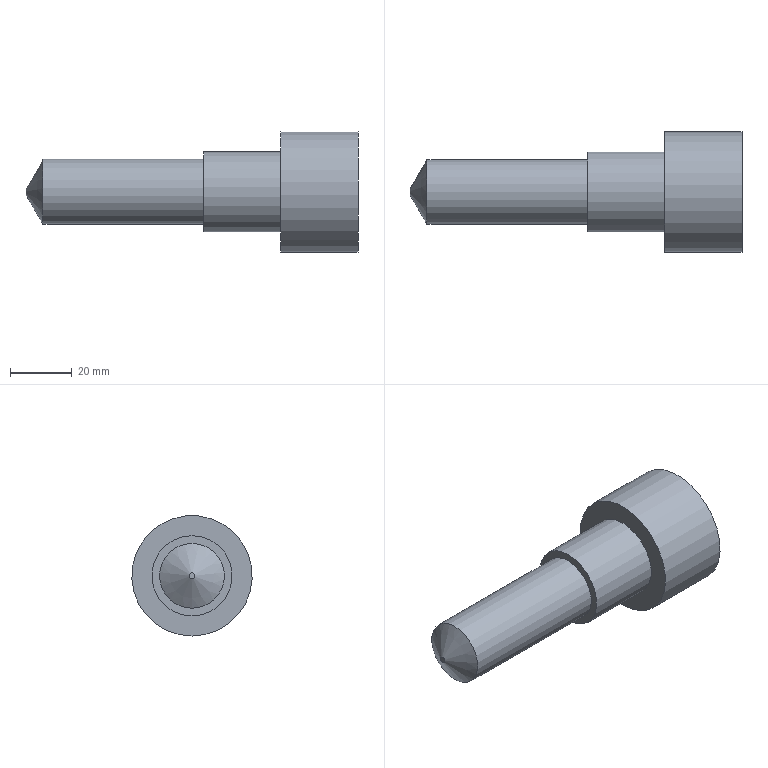Part | STEP file | solid 148 | 1 solid | 8 faces | box 107.5 x 39 x 39 mm | volume 61848 mm3 | plane 4 | cylinder 3 | cone 1 | commonest cylinder face diameters 21 x1 26 x1 39 x1